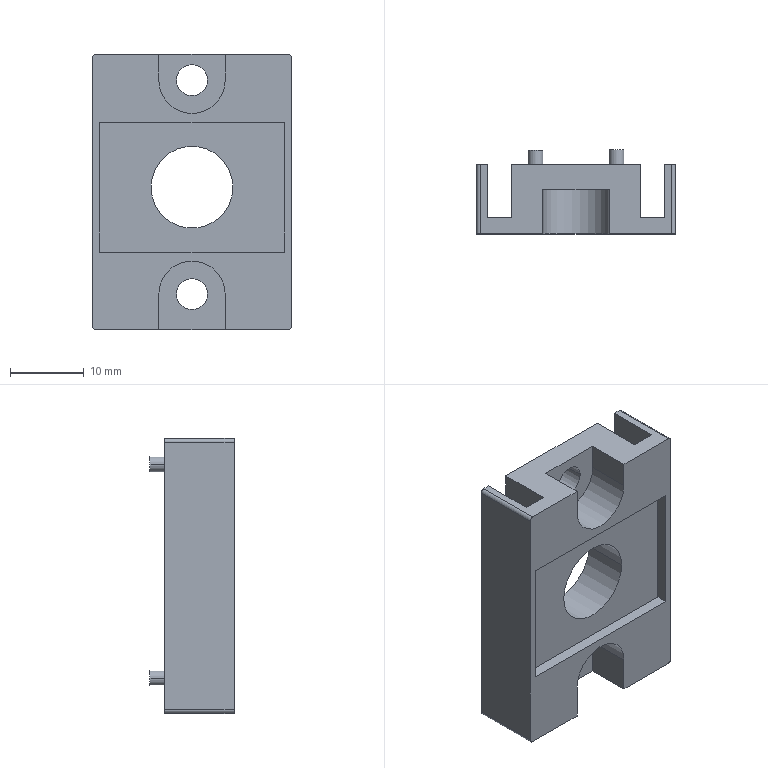Part | STEP file | _X2_751F4E45_X0_MS731-1_X2_8_22 | 1 solid | 59 faces | box 27 x 11.4 x 37.3 mm | volume 4808 mm3 | plane 35 | cylinder 24 | commonest cylinder face diameters 2 x8 1 x4 1.2 x4 4.2 x4 9 x2 11.1 x2